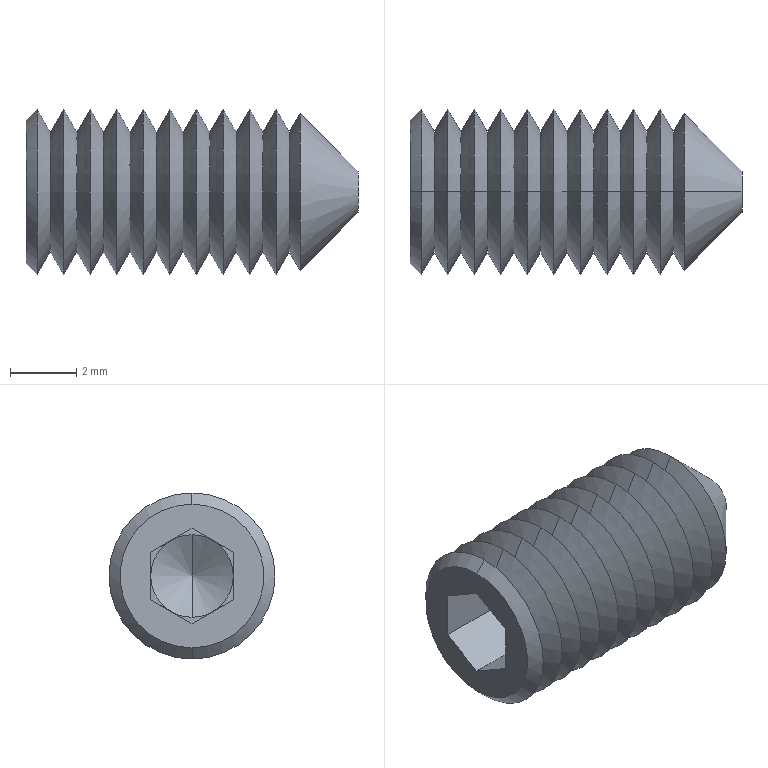Part | STEP file | GB/T 78 M5×10_M5×10 | 1 solid | 60 faces | box 10 x 5 x 5 mm | volume 123.644 mm3 | cone 46 | plane 14
STEP:
#1=CARTESIAN_POINT('',(10.,0.,0.625));
#2=VERTEX_POINT('',#1);
#3=CARTESIAN_POINT('',(10.,0.,-0.625));
#4=VERTEX_POINT('',#3);
#5=CARTESIAN_POINT('',(10.,0.,0.));
#6=DIRECTION('',(-1.,0.,0.));
#7=DIRECTION('',(0.,0.,1.));
#8=AXIS2_PLACEMENT_3D('',#5,#6,#7);
#9=CIRCLE('',#8,0.625);
#10=EDGE_CURVE('',#2,#4,#9,.T.);
#11=ORIENTED_EDGE('',*,*,#10,.T.);
#12=CARTESIAN_POINT('',(8.258,0.,-2.367));
#13=VERTEX_POINT('',#12);
#14=CARTESIAN_POINT('',(10.,0.,-0.625));
#15=DIRECTION('',(-0.7071,0.,-0.7071));
#16=VECTOR('',#15,1000.);
#17=LINE('',#14,#16);
#18=EDGE_CURVE('',#4,#13,#17,.T.);
#19=ORIENTED_EDGE('',*,*,#18,.T.);
#20=CARTESIAN_POINT('',(8.258,0.,2.367));
#21=VERTEX_POINT('',#20);
#22=CARTESIAN_POINT('',(8.258,0.,0.));
#23=DIRECTION('',(-1.,0.,0.));
#24=DIRECTION('',(0.,0.,-1.));
#25=AXIS2_PLACEMENT_3D('',#22,#23,#24);
#26=CIRCLE('',#25,2.367);
#27=EDGE_CURVE('',#21,#13,#26,.T.);
#28=ORIENTED_EDGE('',*,*,#27,.F.);
#29=CARTESIAN_POINT('',(10.,0.,0.625));
#30=DIRECTION('',(-0.7071,0.,0.7071));
#31=VECTOR('',#30,1000.);
#32=LINE('',#29,#31);
#33=EDGE_CURVE('',#2,#21,#32,.T.);
#34=ORIENTED_EDGE('',*,*,#33,.F.);
#35=EDGE_LOOP('',(#11,#19,#28,#34));
#36=FACE_OUTER_BOUND('',#35,.T.);
#37=CARTESIAN_POINT('',(10.,0.,0.));
#38=DIRECTION('',(-1.,0.,0.));
#39=DIRECTION('',(0.,0.,1.));
#40=AXIS2_PLACEMENT_3D('',#37,#38,#39);
#41=CONICAL_SURFACE('',#40,0.625,0.7854);
#42=ADVANCED_FACE('',(#36),#41,.T.);
#43=CARTESIAN_POINT('',(7.931,0.,1.807));
#44=VERTEX_POINT('',#43);
#45=CARTESIAN_POINT('',(7.931,0.,-1.807));
#46=VERTEX_POINT('',#45);
#47=CARTESIAN_POINT('',(7.931,0.,0.));
#48=DIRECTION('',(-1.,0.,0.));
#49=DIRECTION('',(0.,0.,1.));
#50=AXIS2_PLACEMENT_3D('',#47,#48,#49);
#51=CIRCLE('',#50,1.807);
#52=EDGE_CURVE('',#44,#46,#51,.T.);
#53=ORIENTED_EDGE('',*,*,#52,.T.);
#54=CARTESIAN_POINT('',(7.535,0.,-2.5));
#55=VERTEX_POINT('',#54);
#56=CARTESIAN_POINT('',(7.535,0.,-2.5));
#57=DIRECTION('',(-0.4959,0.,-0.8684));
#58=VECTOR('',#57,1000.);
#59=LINE('',#56,#58);
#60=EDGE_CURVE('',#46,#55,#59,.T.);
#61=ORIENTED_EDGE('',*,*,#60,.T.);
#62=CARTESIAN_POINT('',(7.535,0.,2.5));
#63=VERTEX_POINT('',#62);
#64=CARTESIAN_POINT('',(7.535,0.,0.));
#65=DIRECTION('',(-1.,0.,0.));
#66=DIRECTION('',(0.,0.,1.));
#67=AXIS2_PLACEMENT_3D('',#64,#65,#66);
#68=CIRCLE('',#67,2.5);
#69=EDGE_CURVE('',#63,#55,#68,.T.);
#70=ORIENTED_EDGE('',*,*,#69,.F.);
#71=CARTESIAN_POINT('',(7.535,0.,2.5));
#72=DIRECTION('',(-0.4959,0.,0.8684));
#73=VECTOR('',#72,1000.);
#74=LINE('',#71,#73);
#75=EDGE_CURVE('',#44,#63,#74,.T.);
#76=ORIENTED_EDGE('',*,*,#75,.F.);
#77=EDGE_LOOP('',(#53,#61,#70,#76));
#78=FACE_OUTER_BOUND('',#77,.T.);
#79=CARTESIAN_POINT('',(7.535,0.,0.));
#80=DIRECTION('',(-1.,0.,0.));
#81=DIRECTION('',(0.,0.,1.));
#82=AXIS2_PLACEMENT_3D('',#79,#80,#81);
#83=CONICAL_SURFACE('',#82,2.5,1.052);
#84=ADVANCED_FACE('',(#78),#83,.T.);
#85=ORIENTED_EDGE('',*,*,#52,.F.);
#86=CARTESIAN_POINT('',(7.931,0.,1.807));
#87=DIRECTION('',(0.5041,0.,0.8637));
#88=VECTOR('',#87,1000.);
#89=LINE('',#86,#88);
#90=EDGE_CURVE('',#44,#21,#89,.T.);
#91=ORIENTED_EDGE('',*,*,#90,.T.);
#92=ORIENTED_EDGE('',*,*,#27,.T.);
#93=CARTESIAN_POINT('',(7.931,0.,-1.807));
#94=DIRECTION('',(0.5041,0.,-0.8637));
#95=VECTOR('',#94,1000.);
#96=LINE('',#93,#95);
#97=EDGE_CURVE('',#46,#13,#96,.T.);
#98=ORIENTED_EDGE('',*,*,#97,.F.);
#99=EDGE_LOOP('',(#85,#91,#92,#98));
#100=FACE_OUTER_BOUND('',#99,.T.);
#101=CARTESIAN_POINT('',(7.931,0.,0.));
#102=DIRECTION('',(1.,0.,0.));
#103=DIRECTION('',(0.,0.,-1.));
#104=AXIS2_PLACEMENT_3D('',#101,#102,#103);
#105=CONICAL_SURFACE('',#104,1.807,1.043);
#106=ADVANCED_FACE('',(#100),#105,.T.);
#107=CARTESIAN_POINT('',(7.131,0.,1.807));
#108=VERTEX_POINT('',#107);
#109=CARTESIAN_POINT('',(7.131,0.,-1.807));
#110=VERTEX_POINT('',#109);
#111=CARTESIAN_POINT('',(7.131,0.,0.));
#112=DIRECTION('',(-1.,0.,0.));
#113=DIRECTION('',(0.,0.,1.));
#114=AXIS2_PLACEMENT_3D('',#111,#112,#113);
#115=CIRCLE('',#114,1.807);
#116=EDGE_CURVE('',#108,#110,#115,.T.);
#117=ORIENTED_EDGE('',*,*,#116,.F.);
#118=CARTESIAN_POINT('',(7.131,0.,1.807));
#119=DIRECTION('',(0.5041,0.,0.8637));
#120=VECTOR('',#119,1000.);
#121=LINE('',#118,#120);
#122=EDGE_CURVE('',#108,#63,#121,.T.);
#123=ORIENTED_EDGE('',*,*,#122,.T.);
#124=ORIENTED_EDGE('',*,*,#69,.T.);
#125=CARTESIAN_POINT('',(7.131,0.,-1.807));
#126=DIRECTION('',(0.5041,0.,-0.8637));
#127=VECTOR('',#126,1000.);
#128=LINE('',#125,#127);
#129=EDGE_CURVE('',#110,#55,#128,.T.);
#130=ORIENTED_EDGE('',*,*,#129,.F.);
#131=EDGE_LOOP('',(#117,#123,#124,#130));
#132=FACE_OUTER_BOUND('',#131,.T.);
#133=CARTESIAN_POINT('',(7.131,0.,0.));
#134=DIRECTION('',(1.,0.,0.));
#135=DIRECTION('',(0.,0.,-1.));
#136=AXIS2_PLACEMENT_3D('',#133,#134,#135);
#137=CONICAL_SURFACE('',#136,1.807,1.043);
#138=ADVANCED_FACE('',(#132),#137,.T.);
#139=ORIENTED_EDGE('',*,*,#116,.T.);
#140=CARTESIAN_POINT('',(6.735,0.,-2.5));
#141=VERTEX_POINT('',#140);
#142=CARTESIAN_POINT('',(6.735,0.,-2.5));
#143=DIRECTION('',(-0.4959,0.,-0.8684));
#144=VECTOR('',#143,1000.);
#145=LINE('',#142,#144);
#146=EDGE_CURVE('',#110,#141,#145,.T.);
#147=ORIENTED_EDGE('',*,*,#146,.T.);
#148=CARTESIAN_POINT('',(6.735,0.,2.5));
#149=VERTEX_POINT('',#148);
#150=CARTESIAN_POINT('',(6.735,0.,0.));
#151=DIRECTION('',(-1.,0.,0.));
#152=DIRECTION('',(0.,0.,1.));
#153=AXIS2_PLACEMENT_3D('',#150,#151,#152);
#154=CIRCLE('',#153,2.5);
#155=EDGE_CURVE('',#149,#141,#154,.T.);
#156=ORIENTED_EDGE('',*,*,#155,.F.);
#157=CARTESIAN_POINT('',(6.735,0.,2.5));
#158=DIRECTION('',(-0.4959,0.,0.8684));
#159=VECTOR('',#158,1000.);
#160=LINE('',#157,#159);
#161=EDGE_CURVE('',#108,#149,#160,.T.);
#162=ORIENTED_EDGE('',*,*,#161,.F.);
#163=EDGE_LOOP('',(#139,#147,#156,#162));
#164=FACE_OUTER_BOUND('',#163,.T.);
#165=CARTESIAN_POINT('',(6.735,0.,0.));
#166=DIRECTION('',(-1.,0.,0.));
#167=DIRECTION('',(0.,0.,1.));
#168=AXIS2_PLACEMENT_3D('',#165,#166,#167);
#169=CONICAL_SURFACE('',#168,2.5,1.052);
#170=ADVANCED_FACE('',(#164),#169,.T.);
#171=CARTESIAN_POINT('',(6.331,0.,1.807));
#172=VERTEX_POINT('',#171);
#173=CARTESIAN_POINT('',(6.331,0.,-1.807));
#174=VERTEX_POINT('',#173);
#175=CARTESIAN_POINT('',(6.331,0.,0.));
#176=DIRECTION('',(-1.,0.,0.));
#177=DIRECTION('',(0.,0.,1.));
#178=AXIS2_PLACEMENT_3D('',#175,#176,#177);
#179=CIRCLE('',#178,1.807);
#180=EDGE_CURVE('',#172,#174,#179,.T.);
#181=ORIENTED_EDGE('',*,*,#180,.F.);
#182=CARTESIAN_POINT('',(6.331,0.,1.807));
#183=DIRECTION('',(0.5041,0.,0.8637));
#184=VECTOR('',#183,1000.);
#185=LINE('',#182,#184);
#186=EDGE_CURVE('',#172,#149,#185,.T.);
#187=ORIENTED_EDGE('',*,*,#186,.T.);
#188=ORIENTED_EDGE('',*,*,#155,.T.);
#189=CARTESIAN_POINT('',(6.331,0.,-1.807));
#190=DIRECTION('',(0.5041,0.,-0.8637));
#191=VECTOR('',#190,1000.);
#192=LINE('',#189,#191);
#193=EDGE_CURVE('',#174,#141,#192,.T.);
#194=ORIENTED_EDGE('',*,*,#193,.F.);
#195=EDGE_LOOP('',(#181,#187,#188,#194));
#196=FACE_OUTER_BOUND('',#195,.T.);
#197=CARTESIAN_POINT('',(6.331,0.,0.));
#198=DIRECTION('',(1.,0.,0.));
#199=DIRECTION('',(0.,0.,-1.));
#200=AXIS2_PLACEMENT_3D('',#197,#198,#199);
#201=CONICAL_SURFACE('',#200,1.807,1.043);
#202=ADVANCED_FACE('',(#196),#201,.T.);
#203=ORIENTED_EDGE('',*,*,#180,.T.);
#204=CARTESIAN_POINT('',(5.935,0.,-2.5));
#205=VERTEX_POINT('',#204);
#206=CARTESIAN_POINT('',(5.935,0.,-2.5));
#207=DIRECTION('',(-0.4959,0.,-0.8684));
#208=VECTOR('',#207,1000.);
#209=LINE('',#206,#208);
#210=EDGE_CURVE('',#174,#205,#209,.T.);
#211=ORIENTED_EDGE('',*,*,#210,.T.);
#212=CARTESIAN_POINT('',(5.935,0.,2.5));
#213=VERTEX_POINT('',#212);
#214=CARTESIAN_POINT('',(5.935,0.,0.));
#215=DIRECTION('',(-1.,0.,0.));
#216=DIRECTION('',(0.,0.,1.));
#217=AXIS2_PLACEMENT_3D('',#214,#215,#216);
#218=CIRCLE('',#217,2.5);
#219=EDGE_CURVE('',#213,#205,#218,.T.);
#220=ORIENTED_EDGE('',*,*,#219,.F.);
#221=CARTESIAN_POINT('',(5.935,0.,2.5));
#222=DIRECTION('',(-0.4959,0.,0.8684));
#223=VECTOR('',#222,1000.);
#224=LINE('',#221,#223);
#225=EDGE_CURVE('',#172,#213,#224,.T.);
#226=ORIENTED_EDGE('',*,*,#225,.F.);
#227=EDGE_LOOP('',(#203,#211,#220,#226));
#228=FACE_OUTER_BOUND('',#227,.T.);
#229=CARTESIAN_POINT('',(5.935,0.,0.));
#230=DIRECTION('',(-1.,0.,0.));
#231=DIRECTION('',(0.,0.,1.));
#232=AXIS2_PLACEMENT_3D('',#229,#230,#231);
#233=CONICAL_SURFACE('',#232,2.5,1.052);
#234=ADVANCED_FACE('',(#228),#233,.T.);
#235=CARTESIAN_POINT('',(5.531,0.,1.807));
#236=VERTEX_POINT('',#235);
#237=CARTESIAN_POINT('',(5.531,0.,-1.807));
#238=VERTEX_POINT('',#237);
#239=CARTESIAN_POINT('',(5.531,0.,0.));
#240=DIRECTION('',(-1.,0.,0.));
#241=DIRECTION('',(0.,0.,1.));
#242=AXIS2_PLACEMENT_3D('',#239,#240,#241);
#243=CIRCLE('',#242,1.807);
#244=EDGE_CURVE('',#236,#238,#243,.T.);
#245=ORIENTED_EDGE('',*,*,#244,.F.);
#246=CARTESIAN_POINT('',(5.531,0.,1.807));
#247=DIRECTION('',(0.5041,0.,0.8637));
#248=VECTOR('',#247,1000.);
#249=LINE('',#246,#248);
#250=EDGE_CURVE('',#236,#213,#249,.T.);
#251=ORIENTED_EDGE('',*,*,#250,.T.);
#252=ORIENTED_EDGE('',*,*,#219,.T.);
#253=CARTESIAN_POINT('',(5.531,0.,-1.807));
#254=DIRECTION('',(0.5041,0.,-0.8637));
#255=VECTOR('',#254,1000.);
#256=LINE('',#253,#255);
#257=EDGE_CURVE('',#238,#205,#256,.T.);
#258=ORIENTED_EDGE('',*,*,#257,.F.);
#259=EDGE_LOOP('',(#245,#251,#252,#258));
#260=FACE_OUTER_BOUND('',#259,.T.);
#261=CARTESIAN_POINT('',(5.531,0.,0.));
#262=DIRECTION('',(1.,0.,0.));
#263=DIRECTION('',(0.,0.,-1.));
#264=AXIS2_PLACEMENT_3D('',#261,#262,#263);
#265=CONICAL_SURFACE('',#264,1.807,1.043);
#266=ADVANCED_FACE('',(#260),#265,.T.);
#267=ORIENTED_EDGE('',*,*,#244,.T.);
#268=CARTESIAN_POINT('',(5.135,0.,-2.5));
#269=VERTEX_POINT('',#268);
#270=CARTESIAN_POINT('',(5.135,0.,-2.5));
#271=DIRECTION('',(-0.4959,0.,-0.8684));
#272=VECTOR('',#271,1000.);
#273=LINE('',#270,#272);
#274=EDGE_CURVE('',#238,#269,#273,.T.);
#275=ORIENTED_EDGE('',*,*,#274,.T.);
#276=CARTESIAN_POINT('',(5.135,0.,2.5));
#277=VERTEX_POINT('',#276);
#278=CARTESIAN_POINT('',(5.135,0.,0.));
#279=DIRECTION('',(-1.,0.,0.));
#280=DIRECTION('',(0.,0.,1.));
#281=AXIS2_PLACEMENT_3D('',#278,#279,#280);
#282=CIRCLE('',#281,2.5);
#283=EDGE_CURVE('',#277,#269,#282,.T.);
#284=ORIENTED_EDGE('',*,*,#283,.F.);
#285=CARTESIAN_POINT('',(5.135,0.,2.5));
#286=DIRECTION('',(-0.4959,0.,0.8684));
#287=VECTOR('',#286,1000.);
#288=LINE('',#285,#287);
#289=EDGE_CURVE('',#236,#277,#288,.T.);
#290=ORIENTED_EDGE('',*,*,#289,.F.);
#291=EDGE_LOOP('',(#267,#275,#284,#290));
#292=FACE_OUTER_BOUND('',#291,.T.);
#293=CARTESIAN_POINT('',(5.135,0.,0.));
#294=DIRECTION('',(-1.,0.,0.));
#295=DIRECTION('',(0.,0.,1.));
#296=AXIS2_PLACEMENT_3D('',#293,#294,#295);
#297=CONICAL_SURFACE('',#296,2.5,1.052);
#298=ADVANCED_FACE('',(#292),#297,.T.);
#299=CARTESIAN_POINT('',(4.731,0.,1.807));
#300=VERTEX_POINT('',#299);
#301=CARTESIAN_POINT('',(4.731,0.,-1.807));
#302=VERTEX_POINT('',#301);
#303=CARTESIAN_POINT('',(4.731,0.,0.));
#304=DIRECTION('',(-1.,0.,0.));
#305=DIRECTION('',(0.,0.,1.));
#306=AXIS2_PLACEMENT_3D('',#303,#304,#305);
#307=CIRCLE('',#306,1.807);
#308=EDGE_CURVE('',#300,#302,#307,.T.);
#309=ORIENTED_EDGE('',*,*,#308,.F.);
#310=CARTESIAN_POINT('',(4.731,0.,1.807));
#311=DIRECTION('',(0.5041,0.,0.8637));
#312=VECTOR('',#311,1000.);
#313=LINE('',#310,#312);
#314=EDGE_CURVE('',#300,#277,#313,.T.);
#315=ORIENTED_EDGE('',*,*,#314,.T.);
#316=ORIENTED_EDGE('',*,*,#283,.T.);
#317=CARTESIAN_POINT('',(4.731,0.,-1.807));
#318=DIRECTION('',(0.5041,0.,-0.8637));
#319=VECTOR('',#318,1000.);
#320=LINE('',#317,#319);
#321=EDGE_CURVE('',#302,#269,#320,.T.);
#322=ORIENTED_EDGE('',*,*,#321,.F.);
#323=EDGE_LOOP('',(#309,#315,#316,#322));
#324=FACE_OUTER_BOUND('',#323,.T.);
#325=CARTESIAN_POINT('',(4.731,0.,0.));
#326=DIRECTION('',(1.,0.,0.));
#327=DIRECTION('',(0.,0.,-1.));
#328=AXIS2_PLACEMENT_3D('',#325,#326,#327);
#329=CONICAL_SURFACE('',#328,1.807,1.043);
#330=ADVANCED_FACE('',(#324),#329,.T.);
#331=ORIENTED_EDGE('',*,*,#308,.T.);
#332=CARTESIAN_POINT('',(4.335,0.,-2.5));
#333=VERTEX_POINT('',#332);
#334=CARTESIAN_POINT('',(4.335,0.,-2.5));
#335=DIRECTION('',(-0.4959,0.,-0.8684));
#336=VECTOR('',#335,1000.);
#337=LINE('',#334,#336);
#338=EDGE_CURVE('',#302,#333,#337,.T.);
#339=ORIENTED_EDGE('',*,*,#338,.T.);
#340=CARTESIAN_POINT('',(4.335,0.,2.5));
#341=VERTEX_POINT('',#340);
#342=CARTESIAN_POINT('',(4.335,0.,0.));
#343=DIRECTION('',(-1.,0.,0.));
#344=DIRECTION('',(0.,0.,1.));
#345=AXIS2_PLACEMENT_3D('',#342,#343,#344);
#346=CIRCLE('',#345,2.5);
#347=EDGE_CURVE('',#341,#333,#346,.T.);
#348=ORIENTED_EDGE('',*,*,#347,.F.);
#349=CARTESIAN_POINT('',(4.335,0.,2.5));
#350=DIRECTION('',(-0.4959,0.,0.8684));
#351=VECTOR('',#350,1000.);
#352=LINE('',#349,#351);
#353=EDGE_CURVE('',#300,#341,#352,.T.);
#354=ORIENTED_EDGE('',*,*,#353,.F.);
#355=EDGE_LOOP('',(#331,#339,#348,#354));
#356=FACE_OUTER_BOUND('',#355,.T.);
#357=CARTESIAN_POINT('',(4.335,0.,0.));
#358=DIRECTION('',(-1.,0.,0.));
#359=DIRECTION('',(0.,0.,1.));
#360=AXIS2_PLACEMENT_3D('',#357,#358,#359);
#361=CONICAL_SURFACE('',#360,2.5,1.052);
#362=ADVANCED_FACE('',(#356),#361,.T.);
#363=CARTESIAN_POINT('',(3.931,0.,1.807));
#364=VERTEX_POINT('',#363);
#365=CARTESIAN_POINT('',(3.931,0.,-1.807));
#366=VERTEX_POINT('',#365);
#367=CARTESIAN_POINT('',(3.931,0.,0.));
#368=DIRECTION('',(-1.,0.,0.));
#369=DIRECTION('',(0.,0.,1.));
#370=AXIS2_PLACEMENT_3D('',#367,#368,#369);
#371=CIRCLE('',#370,1.807);
#372=EDGE_CURVE('',#364,#366,#371,.T.);
#373=ORIENTED_EDGE('',*,*,#372,.F.);
#374=CARTESIAN_POINT('',(3.931,0.,1.807));
#375=DIRECTION('',(0.5041,0.,0.8637));
#376=VECTOR('',#375,1000.);
#377=LINE('',#374,#376);
#378=EDGE_CURVE('',#364,#341,#377,.T.);
#379=ORIENTED_EDGE('',*,*,#378,.T.);
#380=ORIENTED_EDGE('',*,*,#347,.T.);
#381=CARTESIAN_POINT('',(3.931,0.,-1.807));
#382=DIRECTION('',(0.5041,0.,-0.8637));
#383=VECTOR('',#382,1000.);
#384=LINE('',#381,#383);
#385=EDGE_CURVE('',#366,#333,#384,.T.);
#386=ORIENTED_EDGE('',*,*,#385,.F.);
#387=EDGE_LOOP('',(#373,#379,#380,#386));
#388=FACE_OUTER_BOUND('',#387,.T.);
#389=CARTESIAN_POINT('',(3.931,0.,0.));
#390=DIRECTION('',(1.,0.,0.));
#391=DIRECTION('',(0.,0.,-1.));
#392=AXIS2_PLACEMENT_3D('',#389,#390,#391);
#393=CONICAL_SURFACE('',#392,1.807,1.043);
#394=ADVANCED_FACE('',(#388),#393,.T.);
#395=ORIENTED_EDGE('',*,*,#372,.T.);
#396=CARTESIAN_POINT('',(3.535,0.,-2.5));
#397=VERTEX_POINT('',#396);
#398=CARTESIAN_POINT('',(3.535,0.,-2.5));
#399=DIRECTION('',(-0.4959,0.,-0.8684));
#400=VECTOR('',#399,1000.);
#401=LINE('',#398,#400);
#402=EDGE_CURVE('',#366,#397,#401,.T.);
#403=ORIENTED_EDGE('',*,*,#402,.T.);
#404=CARTESIAN_POINT('',(3.535,0.,2.5));
#405=VERTEX_POINT('',#404);
#406=CARTESIAN_POINT('',(3.535,0.,0.));
#407=DIRECTION('',(-1.,0.,0.));
#408=DIRECTION('',(0.,0.,1.));
#409=AXIS2_PLACEMENT_3D('',#406,#407,#408);
#410=CIRCLE('',#409,2.5);
#411=EDGE_CURVE('',#405,#397,#410,.T.);
#412=ORIENTED_EDGE('',*,*,#411,.F.);
#413=CARTESIAN_POINT('',(3.535,0.,2.5));
#414=DIRECTION('',(-0.4959,0.,0.8684));
#415=VECTOR('',#414,1000.);
#416=LINE('',#413,#415);
#417=EDGE_CURVE('',#364,#405,#416,.T.);
#418=ORIENTED_EDGE('',*,*,#417,.F.);
#419=EDGE_LOOP('',(#395,#403,#412,#418));
#420=FACE_OUTER_BOUND('',#419,.T.);
#421=CARTESIAN_POINT('',(3.535,0.,0.));
#422=DIRECTION('',(-1.,0.,0.));
#423=DIRECTION('',(0.,0.,1.));
#424=AXIS2_PLACEMENT_3D('',#421,#422,#423);
#425=CONICAL_SURFACE('',#424,2.5,1.052);
#426=ADVANCED_FACE('',(#420),#425,.T.);
#427=CARTESIAN_POINT('',(3.131,0.,1.807));
#428=VERTEX_POINT('',#427);
#429=CARTESIAN_POINT('',(3.131,0.,-1.807));
#430=VERTEX_POINT('',#429);
#431=CARTESIAN_POINT('',(3.131,0.,0.));
#432=DIRECTION('',(-1.,0.,0.));
#433=DIRECTION('',(0.,0.,1.));
#434=AXIS2_PLACEMENT_3D('',#431,#432,#433);
#435=CIRCLE('',#434,1.807);
#436=EDGE_CURVE('',#428,#430,#435,.T.);
#437=ORIENTED_EDGE('',*,*,#436,.F.);
#438=CARTESIAN_POINT('',(3.131,0.,1.807));
#439=DIRECTION('',(0.5041,0.,0.8637));
#440=VECTOR('',#439,1000.);
#441=LINE('',#438,#440);
#442=EDGE_CURVE('',#428,#405,#441,.T.);
#443=ORIENTED_EDGE('',*,*,#442,.T.);
#444=ORIENTED_EDGE('',*,*,#411,.T.);
#445=CARTESIAN_POINT('',(3.131,0.,-1.807));
#446=DIRECTION('',(0.5041,0.,-0.8637));
#447=VECTOR('',#446,1000.);
#448=LINE('',#445,#447);
#449=EDGE_CURVE('',#430,#397,#448,.T.);
#450=ORIENTED_EDGE('',*,*,#449,.F.);
#451=EDGE_LOOP('',(#437,#443,#444,#450));
#452=FACE_OUTER_BOUND('',#451,.T.);
#453=CARTESIAN_POINT('',(3.131,0.,0.));
#454=DIRECTION('',(1.,0.,0.));
#455=DIRECTION('',(0.,0.,-1.));
#456=AXIS2_PLACEMENT_3D('',#453,#454,#455);
#457=CONICAL_SURFACE('',#456,1.807,1.043);
#458=ADVANCED_FACE('',(#452),#457,.T.);
#459=ORIENTED_EDGE('',*,*,#436,.T.);
#460=CARTESIAN_POINT('',(2.735,0.,-2.5));
#461=VERTEX_POINT('',#460);
#462=CARTESIAN_POINT('',(2.735,0.,-2.5));
#463=DIRECTION('',(-0.4959,0.,-0.8684));
#464=VECTOR('',#463,1000.);
#465=LINE('',#462,#464);
#466=EDGE_CURVE('',#430,#461,#465,.T.);
#467=ORIENTED_EDGE('',*,*,#466,.T.);
#468=CARTESIAN_POINT('',(2.735,0.,2.5));
#469=VERTEX_POINT('',#468);
#470=CARTESIAN_POINT('',(2.735,0.,0.));
#471=DIRECTION('',(-1.,0.,0.));
#472=DIRECTION('',(0.,0.,1.));
#473=AXIS2_PLACEMENT_3D('',#470,#471,#472);
#474=CIRCLE('',#473,2.5);
#475=EDGE_CURVE('',#469,#461,#474,.T.);
#476=ORIENTED_EDGE('',*,*,#475,.F.);
#477=CARTESIAN_POINT('',(2.735,0.,2.5));
#478=DIRECTION('',(-0.4959,0.,0.8684));
#479=VECTOR('',#478,1000.);
#480=LINE('',#477,#479);
#481=EDGE_CURVE('',#428,#469,#480,.T.);
#482=ORIENTED_EDGE('',*,*,#481,.F.);
#483=EDGE_LOOP('',(#459,#467,#476,#482));
#484=FACE_OUTER_BOUND('',#483,.T.);
#485=CARTESIAN_POINT('',(2.735,0.,0.));
#486=DIRECTION('',(-1.,0.,0.));
#487=DIRECTION('',(0.,0.,1.));
#488=AXIS2_PLACEMENT_3D('',#485,#486,#487);
#489=CONICAL_SURFACE('',#488,2.5,1.052);
#490=ADVANCED_FACE('',(#484),#489,.T.);
#491=CARTESIAN_POINT('',(2.331,0.,1.807));
#492=VERTEX_POINT('',#491);
#493=CARTESIAN_POINT('',(2.331,0.,-1.807));
#494=VERTEX_POINT('',#493);
#495=CARTESIAN_POINT('',(2.331,0.,0.));
#496=DIRECTION('',(-1.,0.,0.));
#497=DIRECTION('',(0.,0.,1.));
#498=AXIS2_PLACEMENT_3D('',#495,#496,#497);
#499=CIRCLE('',#498,1.807);
#500=EDGE_CURVE('',#492,#494,#499,.T.);
#501=ORIENTED_EDGE('',*,*,#500,.F.);
#502=CARTESIAN_POINT('',(2.331,0.,1.807));
#503=DIRECTION('',(0.5041,0.,0.8637));
#504=VECTOR('',#503,1000.);
#505=LINE('',#502,#504);
#506=EDGE_CURVE('',#492,#469,#505,.T.);
#507=ORIENTED_EDGE('',*,*,#506,.T.);
#508=ORIENTED_EDGE('',*,*,#475,.T.);
#509=CARTESIAN_POINT('',(2.331,0.,-1.807));
#510=DIRECTION('',(0.5041,0.,-0.8637));
#511=VECTOR('',#510,1000.);
#512=LINE('',#509,#511);
#513=EDGE_CURVE('',#494,#461,#512,.T.);
#514=ORIENTED_EDGE('',*,*,#513,.F.);
#515=EDGE_LOOP('',(#501,#507,#508,#514));
#516=FACE_OUTER_BOUND('',#515,.T.);
#517=CARTESIAN_POINT('',(2.331,0.,0.));
#518=DIRECTION('',(1.,0.,0.));
#519=DIRECTION('',(0.,0.,-1.));
#520=AXIS2_PLACEMENT_3D('',#517,#518,#519);
#521=CONICAL_SURFACE('',#520,1.807,1.043);
#522=ADVANCED_FACE('',(#516),#521,.T.);
#523=ORIENTED_EDGE('',*,*,#500,.T.);
#524=CARTESIAN_POINT('',(1.935,0.,-2.5));
#525=VERTEX_POINT('',#524);
#526=CARTESIAN_POINT('',(1.935,0.,-2.5));
#527=DIRECTION('',(-0.4959,0.,-0.8684));
#528=VECTOR('',#527,1000.);
#529=LINE('',#526,#528);
#530=EDGE_CURVE('',#494,#525,#529,.T.);
#531=ORIENTED_EDGE('',*,*,#530,.T.);
#532=CARTESIAN_POINT('',(1.935,0.,2.5));
#533=VERTEX_POINT('',#532);
#534=CARTESIAN_POINT('',(1.935,0.,0.));
#535=DIRECTION('',(-1.,0.,0.));
#536=DIRECTION('',(0.,0.,1.));
#537=AXIS2_PLACEMENT_3D('',#534,#535,#536);
#538=CIRCLE('',#537,2.5);
#539=EDGE_CURVE('',#533,#525,#538,.T.);
#540=ORIENTED_EDGE('',*,*,#539,.F.);
#541=CARTESIAN_POINT('',(1.935,0.,2.5));
#542=DIRECTION('',(-0.4959,0.,0.8684));
#543=VECTOR('',#542,1000.);
#544=LINE('',#541,#543);
#545=EDGE_CURVE('',#492,#533,#544,.T.);
#546=ORIENTED_EDGE('',*,*,#545,.F.);
#547=EDGE_LOOP('',(#523,#531,#540,#546));
#548=FACE_OUTER_BOUND('',#547,.T.);
#549=CARTESIAN_POINT('',(1.935,0.,0.));
#550=DIRECTION('',(-1.,0.,0.));
#551=DIRECTION('',(0.,0.,1.));
#552=AXIS2_PLACEMENT_3D('',#549,#550,#551);
#553=CONICAL_SURFACE('',#552,2.5,1.052);
#554=ADVANCED_FACE('',(#548),#553,.T.);
#555=CARTESIAN_POINT('',(1.531,0.,1.807));
#556=VERTEX_POINT('',#555);
#557=CARTESIAN_POINT('',(1.531,0.,-1.807));
#558=VERTEX_POINT('',#557);
#559=CARTESIAN_POINT('',(1.531,0.,0.));
#560=DIRECTION('',(-1.,0.,0.));
#561=DIRECTION('',(0.,0.,1.));
#562=AXIS2_PLACEMENT_3D('',#559,#560,#561);
#563=CIRCLE('',#562,1.807);
#564=EDGE_CURVE('',#556,#558,#563,.T.);
#565=ORIENTED_EDGE('',*,*,#564,.F.);
#566=CARTESIAN_POINT('',(1.531,0.,1.807));
#567=DIRECTION('',(0.5041,0.,0.8637));
#568=VECTOR('',#567,1000.);
#569=LINE('',#566,#568);
#570=EDGE_CURVE('',#556,#533,#569,.T.);
#571=ORIENTED_EDGE('',*,*,#570,.T.);
#572=ORIENTED_EDGE('',*,*,#539,.T.);
#573=CARTESIAN_POINT('',(1.531,0.,-1.807));
#574=DIRECTION('',(0.5041,0.,-0.8637));
#575=VECTOR('',#574,1000.);
#576=LINE('',#573,#575);
#577=EDGE_CURVE('',#558,#525,#576,.T.);
#578=ORIENTED_EDGE('',*,*,#577,.F.);
#579=EDGE_LOOP('',(#565,#571,#572,#578));
#580=FACE_OUTER_BOUND('',#579,.T.);
#581=CARTESIAN_POINT('',(1.531,0.,0.));
#582=DIRECTION('',(1.,0.,0.));
#583=DIRECTION('',(0.,0.,-1.));
#584=AXIS2_PLACEMENT_3D('',#581,#582,#583);
#585=CONICAL_SURFACE('',#584,1.807,1.043);
#586=ADVANCED_FACE('',(#580),#585,.T.);
#587=ORIENTED_EDGE('',*,*,#564,.T.);
#588=CARTESIAN_POINT('',(1.135,0.,-2.5));
#589=VERTEX_POINT('',#588);
#590=CARTESIAN_POINT('',(1.135,0.,-2.5));
#591=DIRECTION('',(-0.4959,0.,-0.8684));
#592=VECTOR('',#591,1000.);
#593=LINE('',#590,#592);
#594=EDGE_CURVE('',#558,#589,#593,.T.);
#595=ORIENTED_EDGE('',*,*,#594,.T.);
#596=CARTESIAN_POINT('',(1.135,0.,2.5));
#597=VERTEX_POINT('',#596);
#598=CARTESIAN_POINT('',(1.135,0.,0.));
#599=DIRECTION('',(-1.,0.,0.));
#600=DIRECTION('',(0.,0.,1.));
#601=AXIS2_PLACEMENT_3D('',#598,#599,#600);
#602=CIRCLE('',#601,2.5);
#603=EDGE_CURVE('',#597,#589,#602,.T.);
#604=ORIENTED_EDGE('',*,*,#603,.F.);
#605=CARTESIAN_POINT('',(1.135,0.,2.5));
#606=DIRECTION('',(-0.4959,0.,0.8684));
#607=VECTOR('',#606,1000.);
#608=LINE('',#605,#607);
#609=EDGE_CURVE('',#556,#597,#608,.T.);
#610=ORIENTED_EDGE('',*,*,#609,.F.);
#611=EDGE_LOOP('',(#587,#595,#604,#610));
#612=FACE_OUTER_BOUND('',#611,.T.);
#613=CARTESIAN_POINT('',(1.135,0.,0.));
#614=DIRECTION('',(-1.,0.,0.));
#615=DIRECTION('',(0.,0.,1.));
#616=AXIS2_PLACEMENT_3D('',#613,#614,#615);
#617=CONICAL_SURFACE('',#616,2.5,1.052);
#618=ADVANCED_FACE('',(#612),#617,.T.);
#619=CARTESIAN_POINT('',(0.7307,0.,1.807));
#620=VERTEX_POINT('',#619);
#621=CARTESIAN_POINT('',(0.7307,0.,-1.807));
#622=VERTEX_POINT('',#621);
#623=CARTESIAN_POINT('',(0.7307,0.,0.));
#624=DIRECTION('',(-1.,0.,0.));
#625=DIRECTION('',(0.,0.,1.));
#626=AXIS2_PLACEMENT_3D('',#623,#624,#625);
#627=CIRCLE('',#626,1.807);
#628=EDGE_CURVE('',#620,#622,#627,.T.);
#629=ORIENTED_EDGE('',*,*,#628,.F.);
#630=CARTESIAN_POINT('',(0.7307,0.,1.807));
#631=DIRECTION('',(0.5041,0.,0.8637));
#632=VECTOR('',#631,1000.);
#633=LINE('',#630,#632);
#634=EDGE_CURVE('',#620,#597,#633,.T.);
#635=ORIENTED_EDGE('',*,*,#634,.T.);
#636=ORIENTED_EDGE('',*,*,#603,.T.);
#637=CARTESIAN_POINT('',(0.7307,0.,-1.807));
#638=DIRECTION('',(0.5041,0.,-0.8637));
#639=VECTOR('',#638,1000.);
#640=LINE('',#637,#639);
#641=EDGE_CURVE('',#622,#589,#640,.T.);
#642=ORIENTED_EDGE('',*,*,#641,.F.);
#643=EDGE_LOOP('',(#629,#635,#636,#642));
#644=FACE_OUTER_BOUND('',#643,.T.);
#645=CARTESIAN_POINT('',(0.7307,0.,0.));
#646=DIRECTION('',(1.,0.,0.));
#647=DIRECTION('',(0.,0.,-1.));
#648=AXIS2_PLACEMENT_3D('',#645,#646,#647);
#649=CONICAL_SURFACE('',#648,1.807,1.043);
#650=ADVANCED_FACE('',(#644),#649,.T.);
#651=ORIENTED_EDGE('',*,*,#628,.T.);
#652=CARTESIAN_POINT('',(0.335,0.,-2.5));
#653=VERTEX_POINT('',#652);
#654=CARTESIAN_POINT('',(0.335,0.,-2.5));
#655=DIRECTION('',(-0.4959,0.,-0.8684));
#656=VECTOR('',#655,1000.);
#657=LINE('',#654,#656);
#658=EDGE_CURVE('',#622,#653,#657,.T.);
#659=ORIENTED_EDGE('',*,*,#658,.T.);
#660=CARTESIAN_POINT('',(0.335,0.,2.5));
#661=VERTEX_POINT('',#660);
#662=CARTESIAN_POINT('',(0.335,0.,0.));
#663=DIRECTION('',(-1.,0.,0.));
#664=DIRECTION('',(0.,0.,1.));
#665=AXIS2_PLACEMENT_3D('',#662,#663,#664);
#666=CIRCLE('',#665,2.5);
#667=EDGE_CURVE('',#661,#653,#666,.T.);
#668=ORIENTED_EDGE('',*,*,#667,.F.);
#669=CARTESIAN_POINT('',(0.335,0.,2.5));
#670=DIRECTION('',(-0.4959,0.,0.8684));
#671=VECTOR('',#670,1000.);
#672=LINE('',#669,#671);
#673=EDGE_CURVE('',#620,#661,#672,.T.);
#674=ORIENTED_EDGE('',*,*,#673,.F.);
#675=EDGE_LOOP('',(#651,#659,#668,#674));
#676=FACE_OUTER_BOUND('',#675,.T.);
#677=CARTESIAN_POINT('',(0.335,0.,0.));
#678=DIRECTION('',(-1.,0.,0.));
#679=DIRECTION('',(0.,0.,1.));
#680=AXIS2_PLACEMENT_3D('',#677,#678,#679);
#681=CONICAL_SURFACE('',#680,2.5,1.052);
#682=ADVANCED_FACE('',(#676),#681,.T.);
#683=CARTESIAN_POINT('',(2.718,0.,0.));
#684=VERTEX_POINT('',#683);
#685=CARTESIAN_POINT('',(2.,0.,1.243));
#686=VERTEX_POINT('',#685);
#687=CARTESIAN_POINT('',(2.718,0.,0.));
#688=DIRECTION('',(-0.5,0.,0.866));
#689=VECTOR('',#688,1000.);
#690=LINE('',#687,#689);
#691=EDGE_CURVE('',#684,#686,#690,.T.);
#692=ORIENTED_EDGE('',*,*,#691,.F.);
#693=CARTESIAN_POINT('',(2.,0.,-1.243));
#694=VERTEX_POINT('',#693);
#695=CARTESIAN_POINT('',(2.718,0.,0.));
#696=DIRECTION('',(-0.5,0.,-0.866));
#697=VECTOR('',#696,1000.);
#698=LINE('',#695,#697);
#699=EDGE_CURVE('',#684,#694,#698,.T.);
#700=ORIENTED_EDGE('',*,*,#699,.T.);
#701=CARTESIAN_POINT('',(2.,-0.6214,-1.076));
#702=VERTEX_POINT('',#701);
#703=CARTESIAN_POINT('',(2.,0.,0.));
#704=DIRECTION('',(-1.,0.,0.));
#705=DIRECTION('',(0.,0.,1.));
#706=AXIS2_PLACEMENT_3D('',#703,#704,#705);
#707=CIRCLE('',#706,1.243);
#708=EDGE_CURVE('',#694,#702,#707,.T.);
#709=ORIENTED_EDGE('',*,*,#708,.T.);
#710=CARTESIAN_POINT('',(2.,-1.243,0.));
#711=VERTEX_POINT('',#710);
#712=CARTESIAN_POINT('',(2.,0.,0.));
#713=DIRECTION('',(-1.,0.,0.));
#714=DIRECTION('',(0.,0.,1.));
#715=AXIS2_PLACEMENT_3D('',#712,#713,#714);
#716=CIRCLE('',#715,1.243);
#717=EDGE_CURVE('',#702,#711,#716,.T.);
#718=ORIENTED_EDGE('',*,*,#717,.T.);
#719=CARTESIAN_POINT('',(2.,-0.6214,1.076));
#720=VERTEX_POINT('',#719);
#721=CARTESIAN_POINT('',(2.,0.,0.));
#722=DIRECTION('',(-1.,0.,0.));
#723=DIRECTION('',(0.,0.,1.));
#724=AXIS2_PLACEMENT_3D('',#721,#722,#723);
#725=CIRCLE('',#724,1.243);
#726=EDGE_CURVE('',#711,#720,#725,.T.);
#727=ORIENTED_EDGE('',*,*,#726,.T.);
#728=CARTESIAN_POINT('',(2.,0.,0.));
#729=DIRECTION('',(-1.,0.,0.));
#730=DIRECTION('',(0.,0.,1.));
#731=AXIS2_PLACEMENT_3D('',#728,#729,#730);
#732=CIRCLE('',#731,1.243);
#733=EDGE_CURVE('',#720,#686,#732,.T.);
#734=ORIENTED_EDGE('',*,*,#733,.T.);
#735=EDGE_LOOP('',(#692,#700,#709,#718,#727,#734));
#736=FACE_OUTER_BOUND('',#735,.T.);
#737=CARTESIAN_POINT('',(-997.282,0.,0.));
#738=DIRECTION('',(-1.,0.,0.));
#739=DIRECTION('',(0.,0.,1.));
#740=AXIS2_PLACEMENT_3D('',#737,#738,#739);
#741=CONICAL_SURFACE('',#740,1732.051,1.047);
#742=ADVANCED_FACE('',(#736),#741,.F.);
#743=CARTESIAN_POINT('',(0.,0.,2.165));
#744=VERTEX_POINT('',#743);
#745=CARTESIAN_POINT('',(0.,0.,-2.165));
#746=VERTEX_POINT('',#745);
#747=CARTESIAN_POINT('',(0.,0.,0.));
#748=DIRECTION('',(-1.,0.,0.));
#749=DIRECTION('',(0.,0.,1.));
#750=AXIS2_PLACEMENT_3D('',#747,#748,#749);
#751=CIRCLE('',#750,2.165);
#752=EDGE_CURVE('',#744,#746,#751,.T.);
#753=ORIENTED_EDGE('',*,*,#752,.F.);
#754=CARTESIAN_POINT('',(0.335,0.,2.5));
#755=DIRECTION('',(0.7071,0.,0.7071));
#756=VECTOR('',#755,1000.);
#757=LINE('',#754,#756);
#758=EDGE_CURVE('',#744,#661,#757,.T.);
#759=ORIENTED_EDGE('',*,*,#758,.T.);
#760=ORIENTED_EDGE('',*,*,#667,.T.);
#761=CARTESIAN_POINT('',(0.335,0.,-2.5));
#762=DIRECTION('',(0.7071,0.,-0.7071));
#763=VECTOR('',#762,1000.);
#764=LINE('',#761,#763);
#765=EDGE_CURVE('',#746,#653,#764,.T.);
#766=ORIENTED_EDGE('',*,*,#765,.F.);
#767=EDGE_LOOP('',(#753,#759,#760,#766));
#768=FACE_OUTER_BOUND('',#767,.T.);
#769=CARTESIAN_POINT('',(0.335,0.,0.));
#770=DIRECTION('',(1.,0.,0.));
#771=DIRECTION('',(0.,0.,-1.));
#772=AXIS2_PLACEMENT_3D('',#769,#770,#771);
#773=CONICAL_SURFACE('',#772,2.5,0.7854);
#774=ADVANCED_FACE('',(#768),#773,.T.);
#775=CARTESIAN_POINT('',(2.,0.6214,1.076));
#776=VERTEX_POINT('',#775);
#777=CARTESIAN_POINT('',(2.,1.243,0.));
#778=VERTEX_POINT('',#777);
#779=CARTESIAN_POINT('',(2.,0.,0.));
#780=DIRECTION('',(-1.,0.,0.));
#781=DIRECTION('',(0.,0.,1.));
#782=AXIS2_PLACEMENT_3D('',#779,#780,#781);
#783=CIRCLE('',#782,1.243);
#784=EDGE_CURVE('',#776,#778,#783,.T.);
#785=ORIENTED_EDGE('',*,*,#784,.F.);
#786=CARTESIAN_POINT('',(2.,1.243,0.7175));
#787=VERTEX_POINT('',#786);
#788=CARTESIAN_POINT('',(2.,0.,1.435));
#789=DIRECTION('',(0.,0.866,-0.5));
#790=VECTOR('',#789,1000.);
#791=LINE('',#788,#790);
#792=EDGE_CURVE('',#776,#787,#791,.T.);
#793=ORIENTED_EDGE('',*,*,#792,.T.);
#794=CARTESIAN_POINT('',(2.,1.243,0.7175));
#795=DIRECTION('',(0.,0.,-1.));
#796=VECTOR('',#795,1000.);
#797=LINE('',#794,#796);
#798=EDGE_CURVE('',#787,#778,#797,.T.);
#799=ORIENTED_EDGE('',*,*,#798,.T.);
#800=EDGE_LOOP('',(#785,#793,#799));
#801=FACE_OUTER_BOUND('',#800,.T.);
#802=CARTESIAN_POINT('',(2.,-1.243,0.7175));
#803=DIRECTION('',(1.,0.,0.));
#804=DIRECTION('',(0.,0.,-1.));
#805=AXIS2_PLACEMENT_3D('',#802,#803,#804);
#806=PLANE('',#805);
#807=ADVANCED_FACE('',(#801),#806,.F.);
#808=CARTESIAN_POINT('',(2.,0.6214,-1.076));
#809=VERTEX_POINT('',#808);
#810=CARTESIAN_POINT('',(2.,0.,0.));
#811=DIRECTION('',(-1.,0.,0.));
#812=DIRECTION('',(0.,0.,1.));
#813=AXIS2_PLACEMENT_3D('',#810,#811,#812);
#814=CIRCLE('',#813,1.243);
#815=EDGE_CURVE('',#778,#809,#814,.T.);
#816=ORIENTED_EDGE('',*,*,#815,.F.);
#817=CARTESIAN_POINT('',(2.,1.243,-0.7175));
#818=VERTEX_POINT('',#817);
#819=CARTESIAN_POINT('',(2.,1.243,0.7175));
#820=DIRECTION('',(0.,0.,-1.));
#821=VECTOR('',#820,1000.);
#822=LINE('',#819,#821);
#823=EDGE_CURVE('',#778,#818,#822,.T.);
#824=ORIENTED_EDGE('',*,*,#823,.T.);
#825=CARTESIAN_POINT('',(2.,1.243,-0.7175));
#826=DIRECTION('',(0.,-0.866,-0.5));
#827=VECTOR('',#826,1000.);
#828=LINE('',#825,#827);
#829=EDGE_CURVE('',#818,#809,#828,.T.);
#830=ORIENTED_EDGE('',*,*,#829,.T.);
#831=EDGE_LOOP('',(#816,#824,#830));
#832=FACE_OUTER_BOUND('',#831,.T.);
#833=CARTESIAN_POINT('',(2.,-1.243,0.7175));
#834=DIRECTION('',(1.,0.,0.));
#835=DIRECTION('',(0.,0.,-1.));
#836=AXIS2_PLACEMENT_3D('',#833,#834,#835);
#837=PLANE('',#836);
#838=ADVANCED_FACE('',(#832),#837,.F.);
#839=CARTESIAN_POINT('',(2.,0.,0.));
#840=DIRECTION('',(-1.,0.,0.));
#841=DIRECTION('',(0.,0.,1.));
#842=AXIS2_PLACEMENT_3D('',#839,#840,#841);
#843=CIRCLE('',#842,1.243);
#844=EDGE_CURVE('',#809,#694,#843,.T.);
#845=ORIENTED_EDGE('',*,*,#844,.F.);
#846=CARTESIAN_POINT('',(2.,0.,-1.435));
#847=VERTEX_POINT('',#846);
#848=CARTESIAN_POINT('',(2.,1.243,-0.7175));
#849=DIRECTION('',(0.,-0.866,-0.5));
#850=VECTOR('',#849,1000.);
#851=LINE('',#848,#850);
#852=EDGE_CURVE('',#809,#847,#851,.T.);
#853=ORIENTED_EDGE('',*,*,#852,.T.);
#854=CARTESIAN_POINT('',(2.,0.,-1.435));
#855=DIRECTION('',(0.,-0.866,0.5));
#856=VECTOR('',#855,1000.);
#857=LINE('',#854,#856);
#858=EDGE_CURVE('',#847,#702,#857,.T.);
#859=ORIENTED_EDGE('',*,*,#858,.T.);
#860=ORIENTED_EDGE('',*,*,#708,.F.);
#861=EDGE_LOOP('',(#845,#853,#859,#860));
#862=FACE_OUTER_BOUND('',#861,.T.);
#863=CARTESIAN_POINT('',(2.,-1.243,0.7175));
#864=DIRECTION('',(1.,0.,0.));
#865=DIRECTION('',(0.,0.,-1.));
#866=AXIS2_PLACEMENT_3D('',#863,#864,#865);
#867=PLANE('',#866);
#868=ADVANCED_FACE('',(#862),#867,.F.);
#869=ORIENTED_EDGE('',*,*,#717,.F.);
#870=CARTESIAN_POINT('',(2.,-1.243,-0.7175));
#871=VERTEX_POINT('',#870);
#872=CARTESIAN_POINT('',(2.,0.,-1.435));
#873=DIRECTION('',(0.,-0.866,0.5));
#874=VECTOR('',#873,1000.);
#875=LINE('',#872,#874);
#876=EDGE_CURVE('',#702,#871,#875,.T.);
#877=ORIENTED_EDGE('',*,*,#876,.T.);
#878=CARTESIAN_POINT('',(2.,-1.243,-0.7175));
#879=DIRECTION('',(0.,0.,1.));
#880=VECTOR('',#879,1000.);
#881=LINE('',#878,#880);
#882=EDGE_CURVE('',#871,#711,#881,.T.);
#883=ORIENTED_EDGE('',*,*,#882,.T.);
#884=EDGE_LOOP('',(#869,#877,#883));
#885=FACE_OUTER_BOUND('',#884,.T.);
#886=CARTESIAN_POINT('',(2.,-1.243,0.7175));
#887=DIRECTION('',(1.,0.,0.));
#888=DIRECTION('',(0.,0.,-1.));
#889=AXIS2_PLACEMENT_3D('',#886,#887,#888);
#890=PLANE('',#889);
#891=ADVANCED_FACE('',(#885),#890,.F.);
#892=ORIENTED_EDGE('',*,*,#726,.F.);
#893=CARTESIAN_POINT('',(2.,-1.243,0.7175));
#894=VERTEX_POINT('',#893);
#895=CARTESIAN_POINT('',(2.,-1.243,-0.7175));
#896=DIRECTION('',(0.,0.,1.));
#897=VECTOR('',#896,1000.);
#898=LINE('',#895,#897);
#899=EDGE_CURVE('',#711,#894,#898,.T.);
#900=ORIENTED_EDGE('',*,*,#899,.T.);
#901=CARTESIAN_POINT('',(2.,-1.243,0.7175));
#902=DIRECTION('',(0.,0.866,0.5));
#903=VECTOR('',#902,1000.);
#904=LINE('',#901,#903);
#905=EDGE_CURVE('',#894,#720,#904,.T.);
#906=ORIENTED_EDGE('',*,*,#905,.T.);
#907=EDGE_LOOP('',(#892,#900,#906));
#908=FACE_OUTER_BOUND('',#907,.T.);
#909=CARTESIAN_POINT('',(2.,-1.243,0.7175));
#910=DIRECTION('',(1.,0.,0.));
#911=DIRECTION('',(0.,0.,-1.));
#912=AXIS2_PLACEMENT_3D('',#909,#910,#911);
#913=PLANE('',#912);
#914=ADVANCED_FACE('',(#908),#913,.F.);
#915=ORIENTED_EDGE('',*,*,#733,.F.);
#916=CARTESIAN_POINT('',(2.,0.,1.435));
#917=VERTEX_POINT('',#916);
#918=CARTESIAN_POINT('',(2.,-1.243,0.7175));
#919=DIRECTION('',(0.,0.866,0.5));
#920=VECTOR('',#919,1000.);
#921=LINE('',#918,#920);
#922=EDGE_CURVE('',#720,#917,#921,.T.);
#923=ORIENTED_EDGE('',*,*,#922,.T.);
#924=CARTESIAN_POINT('',(2.,0.,1.435));
#925=DIRECTION('',(0.,0.866,-0.5));
#926=VECTOR('',#925,1000.);
#927=LINE('',#924,#926);
#928=EDGE_CURVE('',#917,#776,#927,.T.);
#929=ORIENTED_EDGE('',*,*,#928,.T.);
#930=CARTESIAN_POINT('',(2.,0.,0.));
#931=DIRECTION('',(-1.,0.,0.));
#932=DIRECTION('',(0.,0.,1.));
#933=AXIS2_PLACEMENT_3D('',#930,#931,#932);
#934=CIRCLE('',#933,1.243);
#935=EDGE_CURVE('',#686,#776,#934,.T.);
#936=ORIENTED_EDGE('',*,*,#935,.F.);
#937=EDGE_LOOP('',(#915,#923,#929,#936));
#938=FACE_OUTER_BOUND('',#937,.T.);
#939=CARTESIAN_POINT('',(2.,-1.243,0.7175));
#940=DIRECTION('',(1.,0.,0.));
#941=DIRECTION('',(0.,0.,-1.));
#942=AXIS2_PLACEMENT_3D('',#939,#940,#941);
#943=PLANE('',#942);
#944=ADVANCED_FACE('',(#938),#943,.F.);
#945=CARTESIAN_POINT('',(0.,0.,1.435));
#946=VERTEX_POINT('',#945);
#947=CARTESIAN_POINT('',(0.,1.243,0.7175));
#948=VERTEX_POINT('',#947);
#949=CARTESIAN_POINT('',(0.,0.,1.435));
#950=DIRECTION('',(0.,0.866,-0.5));
#951=VECTOR('',#950,1000.);
#952=LINE('',#949,#951);
#953=EDGE_CURVE('',#946,#948,#952,.T.);
#954=ORIENTED_EDGE('',*,*,#953,.F.);
#955=CARTESIAN_POINT('',(0.,-1.243,0.7175));
#956=VERTEX_POINT('',#955);
#957=CARTESIAN_POINT('',(0.,-1.243,0.7175));
#958=DIRECTION('',(0.,0.866,0.5));
#959=VECTOR('',#958,1000.);
#960=LINE('',#957,#959);
#961=EDGE_CURVE('',#956,#946,#960,.T.);
#962=ORIENTED_EDGE('',*,*,#961,.F.);
#963=CARTESIAN_POINT('',(0.,-1.243,-0.7175));
#964=VERTEX_POINT('',#963);
#965=CARTESIAN_POINT('',(0.,-1.243,-0.7175));
#966=DIRECTION('',(0.,0.,1.));
#967=VECTOR('',#966,1000.);
#968=LINE('',#965,#967);
#969=EDGE_CURVE('',#964,#956,#968,.T.);
#970=ORIENTED_EDGE('',*,*,#969,.F.);
#971=CARTESIAN_POINT('',(0.,0.,-1.435));
#972=VERTEX_POINT('',#971);
#973=CARTESIAN_POINT('',(0.,0.,-1.435));
#974=DIRECTION('',(0.,-0.866,0.5));
#975=VECTOR('',#974,1000.);
#976=LINE('',#973,#975);
#977=EDGE_CURVE('',#972,#964,#976,.T.);
#978=ORIENTED_EDGE('',*,*,#977,.F.);
#979=CARTESIAN_POINT('',(0.,1.243,-0.7175));
#980=VERTEX_POINT('',#979);
#981=CARTESIAN_POINT('',(0.,1.243,-0.7175));
#982=DIRECTION('',(0.,-0.866,-0.5));
#983=VECTOR('',#982,1000.);
#984=LINE('',#981,#983);
#985=EDGE_CURVE('',#980,#972,#984,.T.);
#986=ORIENTED_EDGE('',*,*,#985,.F.);
#987=CARTESIAN_POINT('',(0.,1.243,0.7175));
#988=DIRECTION('',(0.,0.,-1.));
#989=VECTOR('',#988,1000.);
#990=LINE('',#987,#989);
#991=EDGE_CURVE('',#948,#980,#990,.T.);
#992=ORIENTED_EDGE('',*,*,#991,.F.);
#993=EDGE_LOOP('',(#954,#962,#970,#978,#986,#992));
#994=FACE_BOUND('',#993,.T.);
#995=CARTESIAN_POINT('',(0.,0.,0.));
#996=DIRECTION('',(-1.,0.,0.));
#997=DIRECTION('',(0.,0.,1.));
#998=AXIS2_PLACEMENT_3D('',#995,#996,#997);
#999=CIRCLE('',#998,2.165);
#1000=EDGE_CURVE('',#746,#744,#999,.T.);
#1001=ORIENTED_EDGE('',*,*,#1000,.T.);
#1002=ORIENTED_EDGE('',*,*,#752,.T.);
#1003=EDGE_LOOP('',(#1001,#1002));
#1004=FACE_OUTER_BOUND('',#1003,.T.);
#1005=CARTESIAN_POINT('',(0.,2.165,0.));
#1006=DIRECTION('',(1.,0.,0.));
#1007=DIRECTION('',(0.,0.,-1.));
#1008=AXIS2_PLACEMENT_3D('',#1005,#1006,#1007);
#1009=PLANE('',#1008);
#1010=ADVANCED_FACE('',(#994,#1004),#1009,.F.);
#1011=ORIENTED_EDGE('',*,*,#758,.F.);
#1012=ORIENTED_EDGE('',*,*,#1000,.F.);
#1013=ORIENTED_EDGE('',*,*,#765,.T.);
#1014=CARTESIAN_POINT('',(0.335,0.,0.));
#1015=DIRECTION('',(-1.,0.,0.));
#1016=DIRECTION('',(0.,0.,1.));
#1017=AXIS2_PLACEMENT_3D('',#1014,#1015,#1016);
#1018=CIRCLE('',#1017,2.5);
#1019=EDGE_CURVE('',#653,#661,#1018,.T.);
#1020=ORIENTED_EDGE('',*,*,#1019,.T.);
#1021=EDGE_LOOP('',(#1011,#1012,#1013,#1020));
#1022=FACE_OUTER_BOUND('',#1021,.T.);
#1023=CARTESIAN_POINT('',(0.335,0.,0.));
#1024=DIRECTION('',(1.,0.,0.));
#1025=DIRECTION('',(0.,0.,-1.));
#1026=AXIS2_PLACEMENT_3D('',#1023,#1024,#1025);
#1027=CONICAL_SURFACE('',#1026,2.5,0.7854);
#1028=ADVANCED_FACE('',(#1022),#1027,.T.);
#1029=ORIENTED_EDGE('',*,*,#961,.T.);
#1030=CARTESIAN_POINT('',(2.,0.,1.435));
#1031=DIRECTION('',(-1.,0.,0.));
#1032=VECTOR('',#1031,1000.);
#1033=LINE('',#1030,#1032);
#1034=EDGE_CURVE('',#917,#946,#1033,.T.);
#1035=ORIENTED_EDGE('',*,*,#1034,.F.);
#1036=ORIENTED_EDGE('',*,*,#922,.F.);
#1037=ORIENTED_EDGE('',*,*,#905,.F.);
#1038=CARTESIAN_POINT('',(2.,-1.243,0.7175));
#1039=DIRECTION('',(-1.,0.,0.));
#1040=VECTOR('',#1039,1000.);
#1041=LINE('',#1038,#1040);
#1042=EDGE_CURVE('',#894,#956,#1041,.T.);
#1043=ORIENTED_EDGE('',*,*,#1042,.T.);
#1044=EDGE_LOOP('',(#1029,#1035,#1036,#1037,#1043));
#1045=FACE_OUTER_BOUND('',#1044,.T.);
#1046=CARTESIAN_POINT('',(2.,-1.243,0.7175));
#1047=DIRECTION('',(0.,-0.5,0.866));
#1048=DIRECTION('',(0.,-0.866,-0.5));
#1049=AXIS2_PLACEMENT_3D('',#1046,#1047,#1048);
#1050=PLANE('',#1049);
#1051=ADVANCED_FACE('',(#1045),#1050,.F.);
#1052=ORIENTED_EDGE('',*,*,#969,.T.);
#1053=ORIENTED_EDGE('',*,*,#1042,.F.);
#1054=ORIENTED_EDGE('',*,*,#899,.F.);
#1055=ORIENTED_EDGE('',*,*,#882,.F.);
#1056=CARTESIAN_POINT('',(2.,-1.243,-0.7175));
#1057=DIRECTION('',(-1.,0.,0.));
#1058=VECTOR('',#1057,1000.);
#1059=LINE('',#1056,#1058);
#1060=EDGE_CURVE('',#871,#964,#1059,.T.);
#1061=ORIENTED_EDGE('',*,*,#1060,.T.);
#1062=EDGE_LOOP('',(#1052,#1053,#1054,#1055,#1061));
#1063=FACE_OUTER_BOUND('',#1062,.T.);
#1064=CARTESIAN_POINT('',(2.,-1.243,-0.7175));
#1065=DIRECTION('',(0.,-1.,0.));
#1066=DIRECTION('',(0.,0.,-1.));
#1067=AXIS2_PLACEMENT_3D('',#1064,#1065,#1066);
#1068=PLANE('',#1067);
#1069=ADVANCED_FACE('',(#1063),#1068,.F.);
#1070=ORIENTED_EDGE('',*,*,#977,.T.);
#1071=ORIENTED_EDGE('',*,*,#1060,.F.);
#1072=ORIENTED_EDGE('',*,*,#876,.F.);
#1073=ORIENTED_EDGE('',*,*,#858,.F.);
#1074=CARTESIAN_POINT('',(2.,0.,-1.435));
#1075=DIRECTION('',(-1.,0.,0.));
#1076=VECTOR('',#1075,1000.);
#1077=LINE('',#1074,#1076);
#1078=EDGE_CURVE('',#847,#972,#1077,.T.);
#1079=ORIENTED_EDGE('',*,*,#1078,.T.);
#1080=EDGE_LOOP('',(#1070,#1071,#1072,#1073,#1079));
#1081=FACE_OUTER_BOUND('',#1080,.T.);
#1082=CARTESIAN_POINT('',(2.,0.,-1.435));
#1083=DIRECTION('',(0.,-0.5,-0.866));
#1084=DIRECTION('',(0.,0.866,-0.5));
#1085=AXIS2_PLACEMENT_3D('',#1082,#1083,#1084);
#1086=PLANE('',#1085);
#1087=ADVANCED_FACE('',(#1081),#1086,.F.);
#1088=ORIENTED_EDGE('',*,*,#985,.T.);
#1089=ORIENTED_EDGE('',*,*,#1078,.F.);
#1090=ORIENTED_EDGE('',*,*,#852,.F.);
#1091=ORIENTED_EDGE('',*,*,#829,.F.);
#1092=CARTESIAN_POINT('',(2.,1.243,-0.7175));
#1093=DIRECTION('',(-1.,0.,0.));
#1094=VECTOR('',#1093,1000.);
#1095=LINE('',#1092,#1094);
#1096=EDGE_CURVE('',#818,#980,#1095,.T.);
#1097=ORIENTED_EDGE('',*,*,#1096,.T.);
#1098=EDGE_LOOP('',(#1088,#1089,#1090,#1091,#1097));
#1099=FACE_OUTER_BOUND('',#1098,.T.);
#1100=CARTESIAN_POINT('',(2.,1.243,-0.7175));
#1101=DIRECTION('',(0.,0.5,-0.866));
#1102=DIRECTION('',(0.,0.866,0.5));
#1103=AXIS2_PLACEMENT_3D('',#1100,#1101,#1102);
#1104=PLANE('',#1103);
#1105=ADVANCED_FACE('',(#1099),#1104,.F.);
#1106=ORIENTED_EDGE('',*,*,#991,.T.);
#1107=ORIENTED_EDGE('',*,*,#1096,.F.);
#1108=ORIENTED_EDGE('',*,*,#823,.F.);
#1109=ORIENTED_EDGE('',*,*,#798,.F.);
#1110=CARTESIAN_POINT('',(2.,1.243,0.7175));
#1111=DIRECTION('',(-1.,0.,0.));
#1112=VECTOR('',#1111,1000.);
#1113=LINE('',#1110,#1112);
#1114=EDGE_CURVE('',#787,#948,#1113,.T.);
#1115=ORIENTED_EDGE('',*,*,#1114,.T.);
#1116=EDGE_LOOP('',(#1106,#1107,#1108,#1109,#1115));
#1117=FACE_OUTER_BOUND('',#1116,.T.);
#1118=CARTESIAN_POINT('',(2.,1.243,0.7175));
#1119=DIRECTION('',(0.,1.,0.));
#1120=DIRECTION('',(0.,0.,1.));
#1121=AXIS2_PLACEMENT_3D('',#1118,#1119,#1120);
#1122=PLANE('',#1121);
#1123=ADVANCED_FACE('',(#1117),#1122,.F.);
#1124=ORIENTED_EDGE('',*,*,#953,.T.);
#1125=ORIENTED_EDGE('',*,*,#1114,.F.);
#1126=ORIENTED_EDGE('',*,*,#792,.F.);
#1127=ORIENTED_EDGE('',*,*,#928,.F.);
#1128=ORIENTED_EDGE('',*,*,#1034,.T.);
#1129=EDGE_LOOP('',(#1124,#1125,#1126,#1127,#1128));
#1130=FACE_OUTER_BOUND('',#1129,.T.);
#1131=CARTESIAN_POINT('',(2.,0.,1.435));
#1132=DIRECTION('',(0.,0.5,0.866));
#1133=DIRECTION('',(0.,-0.866,0.5));
#1134=AXIS2_PLACEMENT_3D('',#1131,#1132,#1133);
#1135=PLANE('',#1134);
#1136=ADVANCED_FACE('',(#1130),#1135,.F.);
#1137=ORIENTED_EDGE('',*,*,#699,.F.);
#1138=ORIENTED_EDGE('',*,*,#691,.T.);
#1139=ORIENTED_EDGE('',*,*,#935,.T.);
#1140=ORIENTED_EDGE('',*,*,#784,.T.);
#1141=ORIENTED_EDGE('',*,*,#815,.T.);
#1142=ORIENTED_EDGE('',*,*,#844,.T.);
#1143=EDGE_LOOP('',(#1137,#1138,#1139,#1140,#1141,#1142));
#1144=FACE_OUTER_BOUND('',#1143,.T.);
#1145=CARTESIAN_POINT('',(-997.282,0.,0.));
#1146=DIRECTION('',(-1.,0.,0.));
#1147=DIRECTION('',(0.,0.,1.));
#1148=AXIS2_PLACEMENT_3D('',#1145,#1146,#1147);
#1149=CONICAL_SURFACE('',#1148,1732.051,1.047);
#1150=ADVANCED_FACE('',(#1144),#1149,.F.);
#1151=ORIENTED_EDGE('',*,*,#658,.F.);
#1152=CARTESIAN_POINT('',(0.7307,0.,0.));
#1153=DIRECTION('',(-1.,0.,0.));
#1154=DIRECTION('',(0.,0.,1.));
#1155=AXIS2_PLACEMENT_3D('',#1152,#1153,#1154);
#1156=CIRCLE('',#1155,1.807);
#1157=EDGE_CURVE('',#622,#620,#1156,.T.);
#1158=ORIENTED_EDGE('',*,*,#1157,.T.);
#1159=ORIENTED_EDGE('',*,*,#673,.T.);
#1160=ORIENTED_EDGE('',*,*,#1019,.F.);
#1161=EDGE_LOOP('',(#1151,#1158,#1159,#1160));
#1162=FACE_OUTER_BOUND('',#1161,.T.);
#1163=CARTESIAN_POINT('',(0.335,0.,0.));
#1164=DIRECTION('',(-1.,0.,0.));
#1165=DIRECTION('',(0.,0.,1.));
#1166=AXIS2_PLACEMENT_3D('',#1163,#1164,#1165);
#1167=CONICAL_SURFACE('',#1166,2.5,1.052);
#1168=ADVANCED_FACE('',(#1162),#1167,.T.);
#1169=ORIENTED_EDGE('',*,*,#634,.F.);
#1170=ORIENTED_EDGE('',*,*,#1157,.F.);
#1171=ORIENTED_EDGE('',*,*,#641,.T.);
#1172=CARTESIAN_POINT('',(1.135,0.,0.));
#1173=DIRECTION('',(-1.,0.,0.));
#1174=DIRECTION('',(0.,0.,1.));
#1175=AXIS2_PLACEMENT_3D('',#1172,#1173,#1174);
#1176=CIRCLE('',#1175,2.5);
#1177=EDGE_CURVE('',#589,#597,#1176,.T.);
#1178=ORIENTED_EDGE('',*,*,#1177,.T.);
#1179=EDGE_LOOP('',(#1169,#1170,#1171,#1178));
#1180=FACE_OUTER_BOUND('',#1179,.T.);
#1181=CARTESIAN_POINT('',(0.7307,0.,0.));
#1182=DIRECTION('',(1.,0.,0.));
#1183=DIRECTION('',(0.,0.,-1.));
#1184=AXIS2_PLACEMENT_3D('',#1181,#1182,#1183);
#1185=CONICAL_SURFACE('',#1184,1.807,1.043);
#1186=ADVANCED_FACE('',(#1180),#1185,.T.);
#1187=ORIENTED_EDGE('',*,*,#594,.F.);
#1188=CARTESIAN_POINT('',(1.531,0.,0.));
#1189=DIRECTION('',(-1.,0.,0.));
#1190=DIRECTION('',(0.,0.,1.));
#1191=AXIS2_PLACEMENT_3D('',#1188,#1189,#1190);
#1192=CIRCLE('',#1191,1.807);
#1193=EDGE_CURVE('',#558,#556,#1192,.T.);
#1194=ORIENTED_EDGE('',*,*,#1193,.T.);
#1195=ORIENTED_EDGE('',*,*,#609,.T.);
#1196=ORIENTED_EDGE('',*,*,#1177,.F.);
#1197=EDGE_LOOP('',(#1187,#1194,#1195,#1196));
#1198=FACE_OUTER_BOUND('',#1197,.T.);
#1199=CARTESIAN_POINT('',(1.135,0.,0.));
#1200=DIRECTION('',(-1.,0.,0.));
#1201=DIRECTION('',(0.,0.,1.));
#1202=AXIS2_PLACEMENT_3D('',#1199,#1200,#1201);
#1203=CONICAL_SURFACE('',#1202,2.5,1.052);
#1204=ADVANCED_FACE('',(#1198),#1203,.T.);
#1205=ORIENTED_EDGE('',*,*,#570,.F.);
#1206=ORIENTED_EDGE('',*,*,#1193,.F.);
#1207=ORIENTED_EDGE('',*,*,#577,.T.);
#1208=CARTESIAN_POINT('',(1.935,0.,0.));
#1209=DIRECTION('',(-1.,0.,0.));
#1210=DIRECTION('',(0.,0.,1.));
#1211=AXIS2_PLACEMENT_3D('',#1208,#1209,#1210);
#1212=CIRCLE('',#1211,2.5);
#1213=EDGE_CURVE('',#525,#533,#1212,.T.);
#1214=ORIENTED_EDGE('',*,*,#1213,.T.);
#1215=EDGE_LOOP('',(#1205,#1206,#1207,#1214));
#1216=FACE_OUTER_BOUND('',#1215,.T.);
#1217=CARTESIAN_POINT('',(1.531,0.,0.));
#1218=DIRECTION('',(1.,0.,0.));
#1219=DIRECTION('',(0.,0.,-1.));
#1220=AXIS2_PLACEMENT_3D('',#1217,#1218,#1219);
#1221=CONICAL_SURFACE('',#1220,1.807,1.043);
#1222=ADVANCED_FACE('',(#1216),#1221,.T.);
#1223=ORIENTED_EDGE('',*,*,#530,.F.);
#1224=CARTESIAN_POINT('',(2.331,0.,0.));
#1225=DIRECTION('',(-1.,0.,0.));
#1226=DIRECTION('',(0.,0.,1.));
#1227=AXIS2_PLACEMENT_3D('',#1224,#1225,#1226);
#1228=CIRCLE('',#1227,1.807);
#1229=EDGE_CURVE('',#494,#492,#1228,.T.);
#1230=ORIENTED_EDGE('',*,*,#1229,.T.);
#1231=ORIENTED_EDGE('',*,*,#545,.T.);
#1232=ORIENTED_EDGE('',*,*,#1213,.F.);
#1233=EDGE_LOOP('',(#1223,#1230,#1231,#1232));
#1234=FACE_OUTER_BOUND('',#1233,.T.);
#1235=CARTESIAN_POINT('',(1.935,0.,0.));
#1236=DIRECTION('',(-1.,0.,0.));
#1237=DIRECTION('',(0.,0.,1.));
#1238=AXIS2_PLACEMENT_3D('',#1235,#1236,#1237);
#1239=CONICAL_SURFACE('',#1238,2.5,1.052);
#1240=ADVANCED_FACE('',(#1234),#1239,.T.);
#1241=ORIENTED_EDGE('',*,*,#506,.F.);
#1242=ORIENTED_EDGE('',*,*,#1229,.F.);
#1243=ORIENTED_EDGE('',*,*,#513,.T.);
#1244=CARTESIAN_POINT('',(2.735,0.,0.));
#1245=DIRECTION('',(-1.,0.,0.));
#1246=DIRECTION('',(0.,0.,1.));
#1247=AXIS2_PLACEMENT_3D('',#1244,#1245,#1246);
#1248=CIRCLE('',#1247,2.5);
#1249=EDGE_CURVE('',#461,#469,#1248,.T.);
#1250=ORIENTED_EDGE('',*,*,#1249,.T.);
#1251=EDGE_LOOP('',(#1241,#1242,#1243,#1250));
#1252=FACE_OUTER_BOUND('',#1251,.T.);
#1253=CARTESIAN_POINT('',(2.331,0.,0.));
#1254=DIRECTION('',(1.,0.,0.));
#1255=DIRECTION('',(0.,0.,-1.));
#1256=AXIS2_PLACEMENT_3D('',#1253,#1254,#1255);
#1257=CONICAL_SURFACE('',#1256,1.807,1.043);
#1258=ADVANCED_FACE('',(#1252),#1257,.T.);
#1259=ORIENTED_EDGE('',*,*,#466,.F.);
#1260=CARTESIAN_POINT('',(3.131,0.,0.));
#1261=DIRECTION('',(-1.,0.,0.));
#1262=DIRECTION('',(0.,0.,1.));
#1263=AXIS2_PLACEMENT_3D('',#1260,#1261,#1262);
#1264=CIRCLE('',#1263,1.807);
#1265=EDGE_CURVE('',#430,#428,#1264,.T.);
#1266=ORIENTED_EDGE('',*,*,#1265,.T.);
#1267=ORIENTED_EDGE('',*,*,#481,.T.);
#1268=ORIENTED_EDGE('',*,*,#1249,.F.);
#1269=EDGE_LOOP('',(#1259,#1266,#1267,#1268));
#1270=FACE_OUTER_BOUND('',#1269,.T.);
#1271=CARTESIAN_POINT('',(2.735,0.,0.));
#1272=DIRECTION('',(-1.,0.,0.));
#1273=DIRECTION('',(0.,0.,1.));
#1274=AXIS2_PLACEMENT_3D('',#1271,#1272,#1273);
#1275=CONICAL_SURFACE('',#1274,2.5,1.052);
#1276=ADVANCED_FACE('',(#1270),#1275,.T.);
#1277=ORIENTED_EDGE('',*,*,#442,.F.);
#1278=ORIENTED_EDGE('',*,*,#1265,.F.);
#1279=ORIENTED_EDGE('',*,*,#449,.T.);
#1280=CARTESIAN_POINT('',(3.535,0.,0.));
#1281=DIRECTION('',(-1.,0.,0.));
#1282=DIRECTION('',(0.,0.,1.));
#1283=AXIS2_PLACEMENT_3D('',#1280,#1281,#1282);
#1284=CIRCLE('',#1283,2.5);
#1285=EDGE_CURVE('',#397,#405,#1284,.T.);
#1286=ORIENTED_EDGE('',*,*,#1285,.T.);
#1287=EDGE_LOOP('',(#1277,#1278,#1279,#1286));
#1288=FACE_OUTER_BOUND('',#1287,.T.);
#1289=CARTESIAN_POINT('',(3.131,0.,0.));
#1290=DIRECTION('',(1.,0.,0.));
#1291=DIRECTION('',(0.,0.,-1.));
#1292=AXIS2_PLACEMENT_3D('',#1289,#1290,#1291);
#1293=CONICAL_SURFACE('',#1292,1.807,1.043);
#1294=ADVANCED_FACE('',(#1288),#1293,.T.);
#1295=ORIENTED_EDGE('',*,*,#402,.F.);
#1296=CARTESIAN_POINT('',(3.931,0.,0.));
#1297=DIRECTION('',(-1.,0.,0.));
#1298=DIRECTION('',(0.,0.,1.));
#1299=AXIS2_PLACEMENT_3D('',#1296,#1297,#1298);
#1300=CIRCLE('',#1299,1.807);
#1301=EDGE_CURVE('',#366,#364,#1300,.T.);
#1302=ORIENTED_EDGE('',*,*,#1301,.T.);
#1303=ORIENTED_EDGE('',*,*,#417,.T.);
#1304=ORIENTED_EDGE('',*,*,#1285,.F.);
#1305=EDGE_LOOP('',(#1295,#1302,#1303,#1304));
#1306=FACE_OUTER_BOUND('',#1305,.T.);
#1307=CARTESIAN_POINT('',(3.535,0.,0.));
#1308=DIRECTION('',(-1.,0.,0.));
#1309=DIRECTION('',(0.,0.,1.));
#1310=AXIS2_PLACEMENT_3D('',#1307,#1308,#1309);
#1311=CONICAL_SURFACE('',#1310,2.5,1.052);
#1312=ADVANCED_FACE('',(#1306),#1311,.T.);
#1313=ORIENTED_EDGE('',*,*,#378,.F.);
#1314=ORIENTED_EDGE('',*,*,#1301,.F.);
#1315=ORIENTED_EDGE('',*,*,#385,.T.);
#1316=CARTESIAN_POINT('',(4.335,0.,0.));
#1317=DIRECTION('',(-1.,0.,0.));
#1318=DIRECTION('',(0.,0.,1.));
#1319=AXIS2_PLACEMENT_3D('',#1316,#1317,#1318);
#1320=CIRCLE('',#1319,2.5);
#1321=EDGE_CURVE('',#333,#341,#1320,.T.);
#1322=ORIENTED_EDGE('',*,*,#1321,.T.);
#1323=EDGE_LOOP('',(#1313,#1314,#1315,#1322));
#1324=FACE_OUTER_BOUND('',#1323,.T.);
#1325=CARTESIAN_POINT('',(3.931,0.,0.));
#1326=DIRECTION('',(1.,0.,0.));
#1327=DIRECTION('',(0.,0.,-1.));
#1328=AXIS2_PLACEMENT_3D('',#1325,#1326,#1327);
#1329=CONICAL_SURFACE('',#1328,1.807,1.043);
#1330=ADVANCED_FACE('',(#1324),#1329,.T.);
#1331=ORIENTED_EDGE('',*,*,#338,.F.);
#1332=CARTESIAN_POINT('',(4.731,0.,0.));
#1333=DIRECTION('',(-1.,0.,0.));
#1334=DIRECTION('',(0.,0.,1.));
#1335=AXIS2_PLACEMENT_3D('',#1332,#1333,#1334);
#1336=CIRCLE('',#1335,1.807);
#1337=EDGE_CURVE('',#302,#300,#1336,.T.);
#1338=ORIENTED_EDGE('',*,*,#1337,.T.);
#1339=ORIENTED_EDGE('',*,*,#353,.T.);
#1340=ORIENTED_EDGE('',*,*,#1321,.F.);
#1341=EDGE_LOOP('',(#1331,#1338,#1339,#1340));
#1342=FACE_OUTER_BOUND('',#1341,.T.);
#1343=CARTESIAN_POINT('',(4.335,0.,0.));
#1344=DIRECTION('',(-1.,0.,0.));
#1345=DIRECTION('',(0.,0.,1.));
#1346=AXIS2_PLACEMENT_3D('',#1343,#1344,#1345);
#1347=CONICAL_SURFACE('',#1346,2.5,1.052);
#1348=ADVANCED_FACE('',(#1342),#1347,.T.);
#1349=ORIENTED_EDGE('',*,*,#314,.F.);
#1350=ORIENTED_EDGE('',*,*,#1337,.F.);
#1351=ORIENTED_EDGE('',*,*,#321,.T.);
#1352=CARTESIAN_POINT('',(5.135,0.,0.));
#1353=DIRECTION('',(-1.,0.,0.));
#1354=DIRECTION('',(0.,0.,1.));
#1355=AXIS2_PLACEMENT_3D('',#1352,#1353,#1354);
#1356=CIRCLE('',#1355,2.5);
#1357=EDGE_CURVE('',#269,#277,#1356,.T.);
#1358=ORIENTED_EDGE('',*,*,#1357,.T.);
#1359=EDGE_LOOP('',(#1349,#1350,#1351,#1358));
#1360=FACE_OUTER_BOUND('',#1359,.T.);
#1361=CARTESIAN_POINT('',(4.731,0.,0.));
#1362=DIRECTION('',(1.,0.,0.));
#1363=DIRECTION('',(0.,0.,-1.));
#1364=AXIS2_PLACEMENT_3D('',#1361,#1362,#1363);
#1365=CONICAL_SURFACE('',#1364,1.807,1.043);
#1366=ADVANCED_FACE('',(#1360),#1365,.T.);
#1367=ORIENTED_EDGE('',*,*,#274,.F.);
#1368=CARTESIAN_POINT('',(5.531,0.,0.));
#1369=DIRECTION('',(-1.,0.,0.));
#1370=DIRECTION('',(0.,0.,1.));
#1371=AXIS2_PLACEMENT_3D('',#1368,#1369,#1370);
#1372=CIRCLE('',#1371,1.807);
#1373=EDGE_CURVE('',#238,#236,#1372,.T.);
#1374=ORIENTED_EDGE('',*,*,#1373,.T.);
#1375=ORIENTED_EDGE('',*,*,#289,.T.);
#1376=ORIENTED_EDGE('',*,*,#1357,.F.);
#1377=EDGE_LOOP('',(#1367,#1374,#1375,#1376));
#1378=FACE_OUTER_BOUND('',#1377,.T.);
#1379=CARTESIAN_POINT('',(5.135,0.,0.));
#1380=DIRECTION('',(-1.,0.,0.));
#1381=DIRECTION('',(0.,0.,1.));
#1382=AXIS2_PLACEMENT_3D('',#1379,#1380,#1381);
#1383=CONICAL_SURFACE('',#1382,2.5,1.052);
#1384=ADVANCED_FACE('',(#1378),#1383,.T.);
#1385=ORIENTED_EDGE('',*,*,#250,.F.);
#1386=ORIENTED_EDGE('',*,*,#1373,.F.);
#1387=ORIENTED_EDGE('',*,*,#257,.T.);
#1388=CARTESIAN_POINT('',(5.935,0.,0.));
#1389=DIRECTION('',(-1.,0.,0.));
#1390=DIRECTION('',(0.,0.,1.));
#1391=AXIS2_PLACEMENT_3D('',#1388,#1389,#1390);
#1392=CIRCLE('',#1391,2.5);
#1393=EDGE_CURVE('',#205,#213,#1392,.T.);
#1394=ORIENTED_EDGE('',*,*,#1393,.T.);
#1395=EDGE_LOOP('',(#1385,#1386,#1387,#1394));
#1396=FACE_OUTER_BOUND('',#1395,.T.);
#1397=CARTESIAN_POINT('',(5.531,0.,0.));
#1398=DIRECTION('',(1.,0.,0.));
#1399=DIRECTION('',(0.,0.,-1.));
#1400=AXIS2_PLACEMENT_3D('',#1397,#1398,#1399);
#1401=CONICAL_SURFACE('',#1400,1.807,1.043);
#1402=ADVANCED_FACE('',(#1396),#1401,.T.);
#1403=ORIENTED_EDGE('',*,*,#210,.F.);
#1404=CARTESIAN_POINT('',(6.331,0.,0.));
#1405=DIRECTION('',(-1.,0.,0.));
#1406=DIRECTION('',(0.,0.,1.));
#1407=AXIS2_PLACEMENT_3D('',#1404,#1405,#1406);
#1408=CIRCLE('',#1407,1.807);
#1409=EDGE_CURVE('',#174,#172,#1408,.T.);
#1410=ORIENTED_EDGE('',*,*,#1409,.T.);
#1411=ORIENTED_EDGE('',*,*,#225,.T.);
#1412=ORIENTED_EDGE('',*,*,#1393,.F.);
#1413=EDGE_LOOP('',(#1403,#1410,#1411,#1412));
#1414=FACE_OUTER_BOUND('',#1413,.T.);
#1415=CARTESIAN_POINT('',(5.935,0.,0.));
#1416=DIRECTION('',(-1.,0.,0.));
#1417=DIRECTION('',(0.,0.,1.));
#1418=AXIS2_PLACEMENT_3D('',#1415,#1416,#1417);
#1419=CONICAL_SURFACE('',#1418,2.5,1.052);
#1420=ADVANCED_FACE('',(#1414),#1419,.T.);
#1421=ORIENTED_EDGE('',*,*,#186,.F.);
#1422=ORIENTED_EDGE('',*,*,#1409,.F.);
#1423=ORIENTED_EDGE('',*,*,#193,.T.);
#1424=CARTESIAN_POINT('',(6.735,0.,0.));
#1425=DIRECTION('',(-1.,0.,0.));
#1426=DIRECTION('',(0.,0.,1.));
#1427=AXIS2_PLACEMENT_3D('',#1424,#1425,#1426);
#1428=CIRCLE('',#1427,2.5);
#1429=EDGE_CURVE('',#141,#149,#1428,.T.);
#1430=ORIENTED_EDGE('',*,*,#1429,.T.);
#1431=EDGE_LOOP('',(#1421,#1422,#1423,#1430));
#1432=FACE_OUTER_BOUND('',#1431,.T.);
#1433=CARTESIAN_POINT('',(6.331,0.,0.));
#1434=DIRECTION('',(1.,0.,0.));
#1435=DIRECTION('',(0.,0.,-1.));
#1436=AXIS2_PLACEMENT_3D('',#1433,#1434,#1435);
#1437=CONICAL_SURFACE('',#1436,1.807,1.043);
#1438=ADVANCED_FACE('',(#1432),#1437,.T.);
#1439=ORIENTED_EDGE('',*,*,#146,.F.);
#1440=CARTESIAN_POINT('',(7.131,0.,0.));
#1441=DIRECTION('',(-1.,0.,0.));
#1442=DIRECTION('',(0.,0.,1.));
#1443=AXIS2_PLACEMENT_3D('',#1440,#1441,#1442);
#1444=CIRCLE('',#1443,1.807);
#1445=EDGE_CURVE('',#110,#108,#1444,.T.);
#1446=ORIENTED_EDGE('',*,*,#1445,.T.);
#1447=ORIENTED_EDGE('',*,*,#161,.T.);
#1448=ORIENTED_EDGE('',*,*,#1429,.F.);
#1449=EDGE_LOOP('',(#1439,#1446,#1447,#1448));
#1450=FACE_OUTER_BOUND('',#1449,.T.);
#1451=CARTESIAN_POINT('',(6.735,0.,0.));
#1452=DIRECTION('',(-1.,0.,0.));
#1453=DIRECTION('',(0.,0.,1.));
#1454=AXIS2_PLACEMENT_3D('',#1451,#1452,#1453);
#1455=CONICAL_SURFACE('',#1454,2.5,1.052);
#1456=ADVANCED_FACE('',(#1450),#1455,.T.);
#1457=ORIENTED_EDGE('',*,*,#122,.F.);
#1458=ORIENTED_EDGE('',*,*,#1445,.F.);
#1459=ORIENTED_EDGE('',*,*,#129,.T.);
#1460=CARTESIAN_POINT('',(7.535,0.,0.));
#1461=DIRECTION('',(-1.,0.,0.));
#1462=DIRECTION('',(0.,0.,1.));
#1463=AXIS2_PLACEMENT_3D('',#1460,#1461,#1462);
#1464=CIRCLE('',#1463,2.5);
#1465=EDGE_CURVE('',#55,#63,#1464,.T.);
#1466=ORIENTED_EDGE('',*,*,#1465,.T.);
#1467=EDGE_LOOP('',(#1457,#1458,#1459,#1466));
#1468=FACE_OUTER_BOUND('',#1467,.T.);
#1469=CARTESIAN_POINT('',(7.131,0.,0.));
#1470=DIRECTION('',(1.,0.,0.));
#1471=DIRECTION('',(0.,0.,-1.));
#1472=AXIS2_PLACEMENT_3D('',#1469,#1470,#1471);
#1473=CONICAL_SURFACE('',#1472,1.807,1.043);
#1474=ADVANCED_FACE('',(#1468),#1473,.T.);
#1475=ORIENTED_EDGE('',*,*,#90,.F.);
#1476=CARTESIAN_POINT('',(7.931,0.,0.));
#1477=DIRECTION('',(-1.,0.,0.));
#1478=DIRECTION('',(0.,0.,1.));
#1479=AXIS2_PLACEMENT_3D('',#1476,#1477,#1478);
#1480=CIRCLE('',#1479,1.807);
#1481=EDGE_CURVE('',#46,#44,#1480,.T.);
#1482=ORIENTED_EDGE('',*,*,#1481,.F.);
#1483=ORIENTED_EDGE('',*,*,#97,.T.);
#1484=CARTESIAN_POINT('',(8.258,0.,0.));
#1485=DIRECTION('',(-1.,0.,0.));
#1486=DIRECTION('',(0.,0.,-1.));
#1487=AXIS2_PLACEMENT_3D('',#1484,#1485,#1486);
#1488=CIRCLE('',#1487,2.367);
#1489=EDGE_CURVE('',#13,#21,#1488,.T.);
#1490=ORIENTED_EDGE('',*,*,#1489,.T.);
#1491=EDGE_LOOP('',(#1475,#1482,#1483,#1490));
#1492=FACE_OUTER_BOUND('',#1491,.T.);
#1493=CARTESIAN_POINT('',(7.931,0.,0.));
#1494=DIRECTION('',(1.,0.,0.));
#1495=DIRECTION('',(0.,0.,-1.));
#1496=AXIS2_PLACEMENT_3D('',#1493,#1494,#1495);
#1497=CONICAL_SURFACE('',#1496,1.807,1.043);
#1498=ADVANCED_FACE('',(#1492),#1497,.T.);
#1499=ORIENTED_EDGE('',*,*,#60,.F.);
#1500=ORIENTED_EDGE('',*,*,#1481,.T.);
#1501=ORIENTED_EDGE('',*,*,#75,.T.);
#1502=ORIENTED_EDGE('',*,*,#1465,.F.);
#1503=EDGE_LOOP('',(#1499,#1500,#1501,#1502));
#1504=FACE_OUTER_BOUND('',#1503,.T.);
#1505=CARTESIAN_POINT('',(7.535,0.,0.));
#1506=DIRECTION('',(-1.,0.,0.));
#1507=DIRECTION('',(0.,0.,1.));
#1508=AXIS2_PLACEMENT_3D('',#1505,#1506,#1507);
#1509=CONICAL_SURFACE('',#1508,2.5,1.052);
#1510=ADVANCED_FACE('',(#1504),#1509,.T.);
#1511=ORIENTED_EDGE('',*,*,#10,.F.);
#1512=CARTESIAN_POINT('',(10.,0.,0.));
#1513=DIRECTION('',(-1.,0.,0.));
#1514=DIRECTION('',(0.,0.,1.));
#1515=AXIS2_PLACEMENT_3D('',#1512,#1513,#1514);
#1516=CIRCLE('',#1515,0.625);
#1517=EDGE_CURVE('',#4,#2,#1516,.T.);
#1518=ORIENTED_EDGE('',*,*,#1517,.F.);
#1519=EDGE_LOOP('',(#1511,#1518));
#1520=FACE_OUTER_BOUND('',#1519,.T.);
#1521=CARTESIAN_POINT('',(10.,0.,0.));
#1522=DIRECTION('',(-1.,0.,0.));
#1523=DIRECTION('',(0.,0.,1.));
#1524=AXIS2_PLACEMENT_3D('',#1521,#1522,#1523);
#1525=PLANE('',#1524);
#1526=ADVANCED_FACE('',(#1520),#1525,.F.);
#1527=ORIENTED_EDGE('',*,*,#18,.F.);
#1528=ORIENTED_EDGE('',*,*,#1517,.T.);
#1529=ORIENTED_EDGE('',*,*,#33,.T.);
#1530=ORIENTED_EDGE('',*,*,#1489,.F.);
#1531=EDGE_LOOP('',(#1527,#1528,#1529,#1530));
#1532=FACE_OUTER_BOUND('',#1531,.T.);
#1533=CARTESIAN_POINT('',(10.,0.,0.));
#1534=DIRECTION('',(-1.,0.,0.));
#1535=DIRECTION('',(0.,0.,1.));
#1536=AXIS2_PLACEMENT_3D('',#1533,#1534,#1535);
#1537=CONICAL_SURFACE('',#1536,0.625,0.7854);
#1538=ADVANCED_FACE('',(#1532),#1537,.T.);
#1539=CLOSED_SHELL('',(#42,#84,#106,#138,#170,#202,#234,#266,#298,#330,#362,#394,#426,#458,#490,#522,#554,#586,#618,#650,#682,#742,#774,#807,#838,#868,#891,#914,#944,#1010,#1028,#1051,#1069,#1087,#1105,#1123,#1136,#1150,#1168,#1186,#1204,#1222,#1240,#1258,#1276,#1294,#1312,#1330,#1348,#1366,#1384,#1402,#1420,#1438,#1456,#1474,#1498,#1510,#1526,#1538));
#1540=MANIFOLD_SOLID_BREP('',#1539);
#1541=CARTESIAN_POINT('',(0.,0.,0.));
#1542=DIRECTION('',(0.,0.,1.));
#1543=DIRECTION('',(1.,0.,0.));
#1544=AXIS2_PLACEMENT_3D('',#1541,#1542,#1543);
#1545=(LENGTH_UNIT()NAMED_UNIT(*)SI_UNIT(.MILLI.,.METRE.));
#1546=UNCERTAINTY_MEASURE_WITH_UNIT(LENGTH_MEASURE(0.00001),#1545,'','');
#1547=(NAMED_UNIT(*)PLANE_ANGLE_UNIT()SI_UNIT($,.RADIAN.));
#1548=(NAMED_UNIT(*)SI_UNIT($,.STERADIAN.)SOLID_ANGLE_UNIT());
#1549=(GEOMETRIC_REPRESENTATION_CONTEXT(3)GLOBAL_UNCERTAINTY_ASSIGNED_CONTEXT((#1546))GLOBAL_UNIT_ASSIGNED_CONTEXT((#1545,#1547,#1548))REPRESENTATION_CONTEXT('',''));
#1550=ADVANCED_BREP_SHAPE_REPRESENTATION('',(#1540,#1544),#1549);